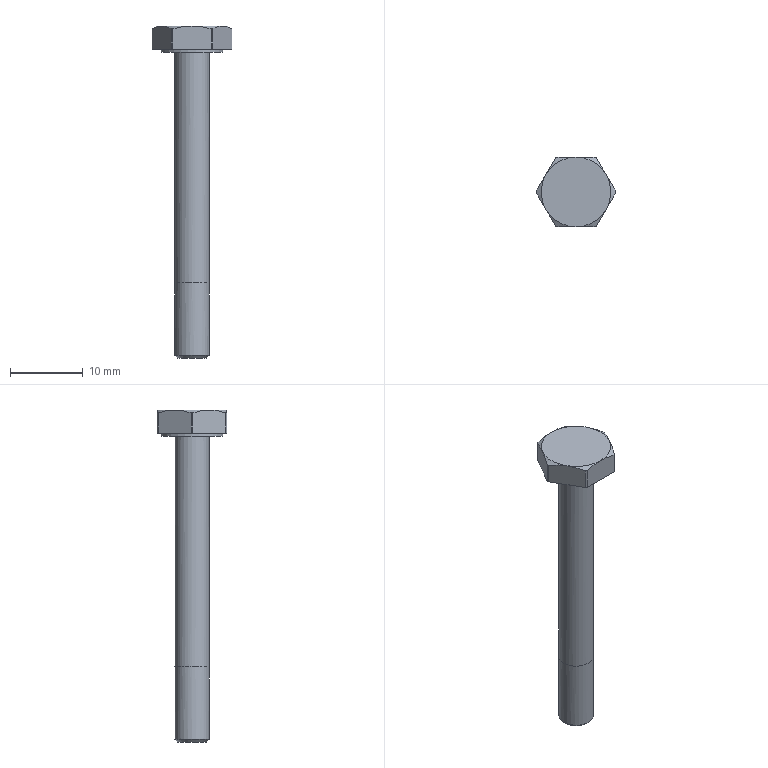Part | NX | features solid 2 | 1 solid | 26 faces | box 10.922 x 9.576 x 45.65 mm | volume 1023 mm3 | plane 10 | cylinder 9 | cone 7 | commonest cylinder face diameters 10.922 x6 4.763 x2 8.509 x1
STEP:
#1=CARTESIAN_POINT('',(-2.381,0.,-3.581));
#2=VERTEX_POINT('',#1);
#3=CARTESIAN_POINT('',(0.,0.,-3.581));
#4=DIRECTION('',(0.,0.,-1.));
#5=DIRECTION('',(-1.,0.,0.));
#6=AXIS2_PLACEMENT_3D('',#3,#4,#5);
#7=CIRCLE('',#6,2.381);
#8=EDGE_CURVE('',#2,#2,#7,.T.);
#9=ORIENTED_EDGE('',*,*,#8,.T.);
#10=EDGE_LOOP('',(#9));
#11=FACE_BOUND('',#10,.T.);
#12=CARTESIAN_POINT('',(-2.381,0.,-35.331));
#13=VERTEX_POINT('',#12);
#14=CARTESIAN_POINT('',(-1.866,1.866,-35.331));
#15=CARTESIAN_POINT('',(-2.639,0.,-35.331));
#16=CARTESIAN_POINT('',(-1.866,-1.866,-35.331));
#17=CARTESIAN_POINT('',(0.,-2.639,-35.331));
#18=CARTESIAN_POINT('',(1.866,-1.866,-35.331));
#19=CARTESIAN_POINT('',(2.639,0.,-35.331));
#20=CARTESIAN_POINT('',(1.866,1.866,-35.331));
#21=CARTESIAN_POINT('',(0.,2.639,-35.331));
#22=CARTESIAN_POINT('',(-1.866,1.866,-35.331));
#23=CARTESIAN_POINT('',(-2.639,0.,-35.331));
#24=CARTESIAN_POINT('',(-1.866,-1.866,-35.331));
#25=B_SPLINE_CURVE_WITH_KNOTS('',3,(#14,#15,#16,#17,#18,#19,#20,#21,#22,#23,#24),.UNSPECIFIED.,.T.,.F.,(1,1,1,1,1,1,1,1,1,1,1,1,1,1,1),(-0.375,-0.25,-0.125,0.,0.125,0.25,0.375,0.5,0.625,0.75,0.875,1.,1.125,1.25,1.375),.UNSPECIFIED.);
#26=EDGE_CURVE('',#13,#13,#25,.T.);
#27=ORIENTED_EDGE('',*,*,#26,.T.);
#28=EDGE_LOOP('',(#27));
#29=FACE_BOUND('',#28,.T.);
#30=CARTESIAN_POINT('',(0.,0.,0.));
#31=DIRECTION('',(0.,0.,-1.));
#32=DIRECTION('',(-1.,0.,0.));
#33=AXIS2_PLACEMENT_3D('',#30,#31,#32);
#34=CYLINDRICAL_SURFACE('',#33,2.381);
#35=ADVANCED_FACE('',(#11,#29),#34,.T.);
#36=CARTESIAN_POINT('',(2.627,4.788,-3.175));
#37=VERTEX_POINT('',#36);
#38=CARTESIAN_POINT('',(2.833,4.669,-3.175));
#39=VERTEX_POINT('',#38);
#40=CARTESIAN_POINT('',(0.,0.,-3.175));
#41=DIRECTION('',(0.,0.,-1.));
#42=DIRECTION('',(-1.,0.,0.));
#43=AXIS2_PLACEMENT_3D('',#40,#41,#42);
#44=CIRCLE('',#43,5.461);
#45=EDGE_CURVE('',#37,#39,#44,.T.);
#46=ORIENTED_EDGE('',*,*,#45,.F.);
#47=CARTESIAN_POINT('',(2.627,4.788,-0.3886));
#48=VERTEX_POINT('',#47);
#49=CARTESIAN_POINT('',(2.627,4.788,0.));
#50=DIRECTION('',(0.,0.,-1.));
#51=VECTOR('',#50,1000.);
#52=LINE('',#49,#51);
#53=EDGE_CURVE('',#37,#48,#52,.F.);
#54=ORIENTED_EDGE('',*,*,#53,.T.);
#55=CARTESIAN_POINT('',(2.833,4.669,-0.3886));
#56=VERTEX_POINT('',#55);
#57=CARTESIAN_POINT('',(0.,0.,-0.3886));
#58=DIRECTION('',(0.,0.,-1.));
#59=DIRECTION('',(-1.,0.,0.));
#60=AXIS2_PLACEMENT_3D('',#57,#58,#59);
#61=CIRCLE('',#60,5.461);
#62=EDGE_CURVE('',#48,#56,#61,.T.);
#63=ORIENTED_EDGE('',*,*,#62,.T.);
#64=CARTESIAN_POINT('',(2.833,4.669,0.));
#65=DIRECTION('',(0.,0.,-1.));
#66=VECTOR('',#65,1000.);
#67=LINE('',#64,#66);
#68=EDGE_CURVE('',#56,#39,#67,.T.);
#69=ORIENTED_EDGE('',*,*,#68,.T.);
#70=EDGE_LOOP('',(#46,#54,#63,#69));
#71=FACE_BOUND('',#70,.T.);
#72=CARTESIAN_POINT('',(0.,0.,0.));
#73=DIRECTION('',(0.,0.,-1.));
#74=DIRECTION('',(-1.,0.,0.));
#75=AXIS2_PLACEMENT_3D('',#72,#73,#74);
#76=CYLINDRICAL_SURFACE('',#75,5.461);
#77=ADVANCED_FACE('',(#71),#76,.T.);
#78=CARTESIAN_POINT('',(-2.833,4.669,-0.3886));
#79=VERTEX_POINT('',#78);
#80=CARTESIAN_POINT('',(-2.627,4.788,-0.3886));
#81=VERTEX_POINT('',#80);
#82=CARTESIAN_POINT('',(0.,0.,-0.3886));
#83=DIRECTION('',(0.,0.,-1.));
#84=DIRECTION('',(-1.,0.,0.));
#85=AXIS2_PLACEMENT_3D('',#82,#83,#84);
#86=CIRCLE('',#85,5.461);
#87=EDGE_CURVE('',#79,#81,#86,.T.);
#88=ORIENTED_EDGE('',*,*,#87,.T.);
#89=CARTESIAN_POINT('',(-2.627,4.788,-3.175));
#90=VERTEX_POINT('',#89);
#91=CARTESIAN_POINT('',(-2.627,4.788,0.));
#92=DIRECTION('',(0.,0.,-1.));
#93=VECTOR('',#92,1000.);
#94=LINE('',#91,#93);
#95=EDGE_CURVE('',#81,#90,#94,.T.);
#96=ORIENTED_EDGE('',*,*,#95,.T.);
#97=CARTESIAN_POINT('',(-2.833,4.669,-3.175));
#98=VERTEX_POINT('',#97);
#99=CARTESIAN_POINT('',(0.,0.,-3.175));
#100=DIRECTION('',(0.,0.,-1.));
#101=DIRECTION('',(-1.,0.,0.));
#102=AXIS2_PLACEMENT_3D('',#99,#100,#101);
#103=CIRCLE('',#102,5.461);
#104=EDGE_CURVE('',#98,#90,#103,.T.);
#105=ORIENTED_EDGE('',*,*,#104,.F.);
#106=CARTESIAN_POINT('',(-2.833,4.669,0.));
#107=DIRECTION('',(0.,0.,-1.));
#108=VECTOR('',#107,1000.);
#109=LINE('',#106,#108);
#110=EDGE_CURVE('',#98,#79,#109,.F.);
#111=ORIENTED_EDGE('',*,*,#110,.T.);
#112=EDGE_LOOP('',(#88,#96,#105,#111));
#113=FACE_BOUND('',#112,.T.);
#114=CARTESIAN_POINT('',(0.,0.,0.));
#115=DIRECTION('',(0.,0.,-1.));
#116=DIRECTION('',(-1.,0.,0.));
#117=AXIS2_PLACEMENT_3D('',#114,#115,#116);
#118=CYLINDRICAL_SURFACE('',#117,5.461);
#119=ADVANCED_FACE('',(#113),#118,.T.);
#120=CARTESIAN_POINT('',(-5.46,-0.1193,-0.3886));
#121=VERTEX_POINT('',#120);
#122=CARTESIAN_POINT('',(-5.46,0.1193,-0.3886));
#123=VERTEX_POINT('',#122);
#124=CARTESIAN_POINT('',(0.,0.,-0.3886));
#125=DIRECTION('',(0.,0.,-1.));
#126=DIRECTION('',(-1.,0.,0.));
#127=AXIS2_PLACEMENT_3D('',#124,#125,#126);
#128=CIRCLE('',#127,5.461);
#129=EDGE_CURVE('',#121,#123,#128,.T.);
#130=ORIENTED_EDGE('',*,*,#129,.T.);
#131=CARTESIAN_POINT('',(-5.46,0.1193,-3.175));
#132=VERTEX_POINT('',#131);
#133=CARTESIAN_POINT('',(-5.46,0.1193,0.));
#134=DIRECTION('',(0.,0.,-1.));
#135=VECTOR('',#134,1000.);
#136=LINE('',#133,#135);
#137=EDGE_CURVE('',#123,#132,#136,.T.);
#138=ORIENTED_EDGE('',*,*,#137,.T.);
#139=CARTESIAN_POINT('',(-5.46,-0.1193,-3.175));
#140=VERTEX_POINT('',#139);
#141=CARTESIAN_POINT('',(0.,0.,-3.175));
#142=DIRECTION('',(0.,0.,-1.));
#143=DIRECTION('',(-1.,0.,0.));
#144=AXIS2_PLACEMENT_3D('',#141,#142,#143);
#145=CIRCLE('',#144,5.461);
#146=EDGE_CURVE('',#140,#132,#145,.T.);
#147=ORIENTED_EDGE('',*,*,#146,.F.);
#148=CARTESIAN_POINT('',(-5.46,-0.1193,0.));
#149=DIRECTION('',(0.,0.,-1.));
#150=VECTOR('',#149,1000.);
#151=LINE('',#148,#150);
#152=EDGE_CURVE('',#140,#121,#151,.F.);
#153=ORIENTED_EDGE('',*,*,#152,.T.);
#154=EDGE_LOOP('',(#130,#138,#147,#153));
#155=FACE_BOUND('',#154,.T.);
#156=CARTESIAN_POINT('',(0.,0.,0.));
#157=DIRECTION('',(0.,0.,-1.));
#158=DIRECTION('',(-1.,0.,0.));
#159=AXIS2_PLACEMENT_3D('',#156,#157,#158);
#160=CYLINDRICAL_SURFACE('',#159,5.461);
#161=ADVANCED_FACE('',(#155),#160,.T.);
#162=CARTESIAN_POINT('',(-2.627,-4.788,-0.3886));
#163=VERTEX_POINT('',#162);
#164=CARTESIAN_POINT('',(-2.833,-4.669,-0.3886));
#165=VERTEX_POINT('',#164);
#166=CARTESIAN_POINT('',(0.,0.,-0.3886));
#167=DIRECTION('',(0.,0.,-1.));
#168=DIRECTION('',(-1.,0.,0.));
#169=AXIS2_PLACEMENT_3D('',#166,#167,#168);
#170=CIRCLE('',#169,5.461);
#171=EDGE_CURVE('',#163,#165,#170,.T.);
#172=ORIENTED_EDGE('',*,*,#171,.T.);
#173=CARTESIAN_POINT('',(-2.833,-4.669,-3.175));
#174=VERTEX_POINT('',#173);
#175=CARTESIAN_POINT('',(-2.833,-4.669,0.));
#176=DIRECTION('',(0.,0.,-1.));
#177=VECTOR('',#176,1000.);
#178=LINE('',#175,#177);
#179=EDGE_CURVE('',#165,#174,#178,.T.);
#180=ORIENTED_EDGE('',*,*,#179,.T.);
#181=CARTESIAN_POINT('',(-2.627,-4.788,-3.175));
#182=VERTEX_POINT('',#181);
#183=CARTESIAN_POINT('',(0.,0.,-3.175));
#184=DIRECTION('',(0.,0.,-1.));
#185=DIRECTION('',(-1.,0.,0.));
#186=AXIS2_PLACEMENT_3D('',#183,#184,#185);
#187=CIRCLE('',#186,5.461);
#188=EDGE_CURVE('',#182,#174,#187,.T.);
#189=ORIENTED_EDGE('',*,*,#188,.F.);
#190=CARTESIAN_POINT('',(-2.627,-4.788,0.));
#191=DIRECTION('',(0.,0.,-1.));
#192=VECTOR('',#191,1000.);
#193=LINE('',#190,#192);
#194=EDGE_CURVE('',#182,#163,#193,.F.);
#195=ORIENTED_EDGE('',*,*,#194,.T.);
#196=EDGE_LOOP('',(#172,#180,#189,#195));
#197=FACE_BOUND('',#196,.T.);
#198=CARTESIAN_POINT('',(0.,0.,0.));
#199=DIRECTION('',(0.,0.,-1.));
#200=DIRECTION('',(-1.,0.,0.));
#201=AXIS2_PLACEMENT_3D('',#198,#199,#200);
#202=CYLINDRICAL_SURFACE('',#201,5.461);
#203=ADVANCED_FACE('',(#197),#202,.T.);
#204=CARTESIAN_POINT('',(2.833,-4.669,-0.3886));
#205=VERTEX_POINT('',#204);
#206=CARTESIAN_POINT('',(2.627,-4.788,-0.3886));
#207=VERTEX_POINT('',#206);
#208=CARTESIAN_POINT('',(0.,0.,-0.3886));
#209=DIRECTION('',(0.,0.,-1.));
#210=DIRECTION('',(-1.,0.,0.));
#211=AXIS2_PLACEMENT_3D('',#208,#209,#210);
#212=CIRCLE('',#211,5.461);
#213=EDGE_CURVE('',#205,#207,#212,.T.);
#214=ORIENTED_EDGE('',*,*,#213,.T.);
#215=CARTESIAN_POINT('',(2.627,-4.788,-3.175));
#216=VERTEX_POINT('',#215);
#217=CARTESIAN_POINT('',(2.627,-4.788,0.));
#218=DIRECTION('',(0.,0.,-1.));
#219=VECTOR('',#218,1000.);
#220=LINE('',#217,#219);
#221=EDGE_CURVE('',#207,#216,#220,.T.);
#222=ORIENTED_EDGE('',*,*,#221,.T.);
#223=CARTESIAN_POINT('',(2.833,-4.669,-3.175));
#224=VERTEX_POINT('',#223);
#225=CARTESIAN_POINT('',(0.,0.,-3.175));
#226=DIRECTION('',(0.,0.,-1.));
#227=DIRECTION('',(-1.,0.,0.));
#228=AXIS2_PLACEMENT_3D('',#225,#226,#227);
#229=CIRCLE('',#228,5.461);
#230=EDGE_CURVE('',#224,#216,#229,.T.);
#231=ORIENTED_EDGE('',*,*,#230,.F.);
#232=CARTESIAN_POINT('',(2.833,-4.669,0.));
#233=DIRECTION('',(0.,0.,-1.));
#234=VECTOR('',#233,1000.);
#235=LINE('',#232,#234);
#236=EDGE_CURVE('',#224,#205,#235,.F.);
#237=ORIENTED_EDGE('',*,*,#236,.T.);
#238=EDGE_LOOP('',(#214,#222,#231,#237));
#239=FACE_BOUND('',#238,.T.);
#240=CARTESIAN_POINT('',(0.,0.,0.));
#241=DIRECTION('',(0.,0.,-1.));
#242=DIRECTION('',(-1.,0.,0.));
#243=AXIS2_PLACEMENT_3D('',#240,#241,#242);
#244=CYLINDRICAL_SURFACE('',#243,5.461);
#245=ADVANCED_FACE('',(#239),#244,.T.);
#246=ORIENTED_EDGE('',*,*,#62,.F.);
#247=CARTESIAN_POINT('',(0.,4.788,0.));
#248=VERTEX_POINT('',#247);
#249=CARTESIAN_POINT('',(0.,4.788,0.));
#250=CARTESIAN_POINT('',(0.8868,4.788,0.));
#251=CARTESIAN_POINT('',(1.776,4.788,-0.1525));
#252=CARTESIAN_POINT('',(2.627,4.788,-0.3886));
#253=B_SPLINE_CURVE_WITH_KNOTS('',3,(#249,#250,#251,#252),.UNSPECIFIED.,.F.,.F.,(4,4),(0.007722,0.01038),.UNSPECIFIED.);
#254=EDGE_CURVE('',#48,#248,#253,.F.);
#255=ORIENTED_EDGE('',*,*,#254,.T.);
#256=CARTESIAN_POINT('',(4.146,2.394,0.));
#257=VERTEX_POINT('',#256);
#258=CARTESIAN_POINT('',(0.,0.,0.));
#259=DIRECTION('',(0.,0.,-1.));
#260=DIRECTION('',(-1.,0.,0.));
#261=AXIS2_PLACEMENT_3D('',#258,#259,#260);
#262=CIRCLE('',#261,4.788);
#263=EDGE_CURVE('',#248,#257,#262,.T.);
#264=ORIENTED_EDGE('',*,*,#263,.T.);
#265=CARTESIAN_POINT('',(4.146,2.394,0.));
#266=CARTESIAN_POINT('',(3.703,3.163,0.));
#267=CARTESIAN_POINT('',(3.262,3.925,-0.1503));
#268=CARTESIAN_POINT('',(2.833,4.669,-0.3886));
#269=B_SPLINE_CURVE_WITH_KNOTS('',3,(#265,#266,#267,#268),.UNSPECIFIED.,.F.,.F.,(4,4),(0.002655,0.005296),.UNSPECIFIED.);
#270=EDGE_CURVE('',#257,#56,#269,.T.);
#271=ORIENTED_EDGE('',*,*,#270,.T.);
#272=EDGE_LOOP('',(#246,#255,#264,#271));
#273=FACE_BOUND('',#272,.T.);
#274=CARTESIAN_POINT('',(0.,0.,-0.3886));
#275=DIRECTION('',(0.,0.,-1.));
#276=DIRECTION('',(-1.,0.,0.));
#277=AXIS2_PLACEMENT_3D('',#274,#275,#276);
#278=CONICAL_SURFACE('',#277,5.461,1.047);
#279=ADVANCED_FACE('',(#273),#278,.T.);
#280=CARTESIAN_POINT('',(-4.146,2.394,0.));
#281=VERTEX_POINT('',#280);
#282=CARTESIAN_POINT('',(0.,0.,0.));
#283=DIRECTION('',(0.,0.,-1.));
#284=DIRECTION('',(-1.,0.,0.));
#285=AXIS2_PLACEMENT_3D('',#282,#283,#284);
#286=CIRCLE('',#285,4.788);
#287=EDGE_CURVE('',#281,#248,#286,.T.);
#288=ORIENTED_EDGE('',*,*,#287,.T.);
#289=CARTESIAN_POINT('',(-2.627,4.788,-0.3886));
#290=CARTESIAN_POINT('',(-1.77,4.788,-0.1508));
#291=CARTESIAN_POINT('',(-0.8866,4.788,0.));
#292=CARTESIAN_POINT('',(0.,4.788,0.));
#293=B_SPLINE_CURVE_WITH_KNOTS('',3,(#289,#290,#291,#292),.UNSPECIFIED.,.F.,.F.,(4,4),(0.005068,0.007722),.UNSPECIFIED.);
#294=EDGE_CURVE('',#248,#81,#293,.F.);
#295=ORIENTED_EDGE('',*,*,#294,.T.);
#296=ORIENTED_EDGE('',*,*,#87,.F.);
#297=CARTESIAN_POINT('',(-2.833,4.669,-0.3886));
#298=CARTESIAN_POINT('',(-3.264,3.923,-0.1495));
#299=CARTESIAN_POINT('',(-3.7,3.167,0.));
#300=CARTESIAN_POINT('',(-4.146,2.394,0.));
#301=B_SPLINE_CURVE_WITH_KNOTS('',3,(#297,#298,#299,#300),.UNSPECIFIED.,.F.,.F.,(4,4),(0.00000074,0.002655),.UNSPECIFIED.);
#302=EDGE_CURVE('',#79,#281,#301,.T.);
#303=ORIENTED_EDGE('',*,*,#302,.T.);
#304=EDGE_LOOP('',(#288,#295,#296,#303));
#305=FACE_BOUND('',#304,.T.);
#306=CARTESIAN_POINT('',(0.,0.,-0.3886));
#307=DIRECTION('',(0.,0.,-1.));
#308=DIRECTION('',(-1.,0.,0.));
#309=AXIS2_PLACEMENT_3D('',#306,#307,#308);
#310=CONICAL_SURFACE('',#309,5.461,1.047);
#311=ADVANCED_FACE('',(#305),#310,.T.);
#312=CARTESIAN_POINT('',(-4.146,-2.394,0.));
#313=VERTEX_POINT('',#312);
#314=CARTESIAN_POINT('',(0.,0.,0.));
#315=DIRECTION('',(0.,0.,-1.));
#316=DIRECTION('',(-1.,0.,0.));
#317=AXIS2_PLACEMENT_3D('',#314,#315,#316);
#318=CIRCLE('',#317,4.788);
#319=EDGE_CURVE('',#313,#281,#318,.T.);
#320=ORIENTED_EDGE('',*,*,#319,.T.);
#321=CARTESIAN_POINT('',(-4.146,2.394,0.));
#322=CARTESIAN_POINT('',(-4.59,1.625,0.));
#323=CARTESIAN_POINT('',(-5.031,0.8625,-0.1503));
#324=CARTESIAN_POINT('',(-5.46,0.1193,-0.3886));
#325=B_SPLINE_CURVE_WITH_KNOTS('',3,(#321,#322,#323,#324),.UNSPECIFIED.,.F.,.F.,(4,4),(0.002655,0.005296),.UNSPECIFIED.);
#326=EDGE_CURVE('',#281,#123,#325,.T.);
#327=ORIENTED_EDGE('',*,*,#326,.T.);
#328=ORIENTED_EDGE('',*,*,#129,.F.);
#329=CARTESIAN_POINT('',(-5.46,-0.1193,-0.3886));
#330=CARTESIAN_POINT('',(-5.029,-0.8651,-0.1495));
#331=CARTESIAN_POINT('',(-4.593,-1.621,0.));
#332=CARTESIAN_POINT('',(-4.146,-2.394,0.));
#333=B_SPLINE_CURVE_WITH_KNOTS('',3,(#329,#330,#331,#332),.UNSPECIFIED.,.F.,.F.,(4,4),(0.00000074,0.002655),.UNSPECIFIED.);
#334=EDGE_CURVE('',#121,#313,#333,.T.);
#335=ORIENTED_EDGE('',*,*,#334,.T.);
#336=EDGE_LOOP('',(#320,#327,#328,#335));
#337=FACE_BOUND('',#336,.T.);
#338=CARTESIAN_POINT('',(0.,0.,-0.3886));
#339=DIRECTION('',(0.,0.,-1.));
#340=DIRECTION('',(-1.,0.,0.));
#341=AXIS2_PLACEMENT_3D('',#338,#339,#340);
#342=CONICAL_SURFACE('',#341,5.461,1.047);
#343=ADVANCED_FACE('',(#337),#342,.T.);
#344=CARTESIAN_POINT('',(0.,-4.788,0.));
#345=VERTEX_POINT('',#344);
#346=CARTESIAN_POINT('',(0.,0.,0.));
#347=DIRECTION('',(0.,0.,-1.));
#348=DIRECTION('',(-1.,0.,0.));
#349=AXIS2_PLACEMENT_3D('',#346,#347,#348);
#350=CIRCLE('',#349,4.788);
#351=EDGE_CURVE('',#345,#313,#350,.T.);
#352=ORIENTED_EDGE('',*,*,#351,.T.);
#353=CARTESIAN_POINT('',(-4.146,-2.394,0.));
#354=CARTESIAN_POINT('',(-3.703,-3.163,0.));
#355=CARTESIAN_POINT('',(-3.262,-3.925,-0.1503));
#356=CARTESIAN_POINT('',(-2.833,-4.669,-0.3886));
#357=B_SPLINE_CURVE_WITH_KNOTS('',3,(#353,#354,#355,#356),.UNSPECIFIED.,.F.,.F.,(4,4),(0.002655,0.005296),.UNSPECIFIED.);
#358=EDGE_CURVE('',#313,#165,#357,.T.);
#359=ORIENTED_EDGE('',*,*,#358,.T.);
#360=ORIENTED_EDGE('',*,*,#171,.F.);
#361=CARTESIAN_POINT('',(-2.627,-4.788,-0.3886));
#362=CARTESIAN_POINT('',(-1.77,-4.788,-0.1508));
#363=CARTESIAN_POINT('',(-0.8866,-4.788,0.));
#364=CARTESIAN_POINT('',(0.,-4.788,0.));
#365=B_SPLINE_CURVE_WITH_KNOTS('',3,(#361,#362,#363,#364),.UNSPECIFIED.,.F.,.F.,(4,4),(0.005068,0.007722),.UNSPECIFIED.);
#366=EDGE_CURVE('',#163,#345,#365,.T.);
#367=ORIENTED_EDGE('',*,*,#366,.T.);
#368=EDGE_LOOP('',(#352,#359,#360,#367));
#369=FACE_BOUND('',#368,.T.);
#370=CARTESIAN_POINT('',(0.,0.,-0.3886));
#371=DIRECTION('',(0.,0.,-1.));
#372=DIRECTION('',(-1.,0.,0.));
#373=AXIS2_PLACEMENT_3D('',#370,#371,#372);
#374=CONICAL_SURFACE('',#373,5.461,1.047);
#375=ADVANCED_FACE('',(#369),#374,.T.);
#376=CARTESIAN_POINT('',(4.146,-2.394,0.));
#377=VERTEX_POINT('',#376);
#378=CARTESIAN_POINT('',(0.,0.,0.));
#379=DIRECTION('',(0.,0.,-1.));
#380=DIRECTION('',(-1.,0.,0.));
#381=AXIS2_PLACEMENT_3D('',#378,#379,#380);
#382=CIRCLE('',#381,4.788);
#383=EDGE_CURVE('',#377,#345,#382,.T.);
#384=ORIENTED_EDGE('',*,*,#383,.T.);
#385=CARTESIAN_POINT('',(0.,-4.788,0.));
#386=CARTESIAN_POINT('',(0.8868,-4.788,0.));
#387=CARTESIAN_POINT('',(1.776,-4.788,-0.1525));
#388=CARTESIAN_POINT('',(2.627,-4.788,-0.3886));
#389=B_SPLINE_CURVE_WITH_KNOTS('',3,(#385,#386,#387,#388),.UNSPECIFIED.,.F.,.F.,(4,4),(0.007722,0.01038),.UNSPECIFIED.);
#390=EDGE_CURVE('',#345,#207,#389,.T.);
#391=ORIENTED_EDGE('',*,*,#390,.T.);
#392=ORIENTED_EDGE('',*,*,#213,.F.);
#393=CARTESIAN_POINT('',(2.833,-4.669,-0.3886));
#394=CARTESIAN_POINT('',(3.264,-3.923,-0.1495));
#395=CARTESIAN_POINT('',(3.7,-3.167,0.));
#396=CARTESIAN_POINT('',(4.146,-2.394,0.));
#397=B_SPLINE_CURVE_WITH_KNOTS('',3,(#393,#394,#395,#396),.UNSPECIFIED.,.F.,.F.,(4,4),(0.00000074,0.002655),.UNSPECIFIED.);
#398=EDGE_CURVE('',#205,#377,#397,.T.);
#399=ORIENTED_EDGE('',*,*,#398,.T.);
#400=EDGE_LOOP('',(#384,#391,#392,#399));
#401=FACE_BOUND('',#400,.T.);
#402=CARTESIAN_POINT('',(0.,0.,-0.3886));
#403=DIRECTION('',(0.,0.,-1.));
#404=DIRECTION('',(-1.,0.,0.));
#405=AXIS2_PLACEMENT_3D('',#402,#403,#404);
#406=CONICAL_SURFACE('',#405,5.461,1.047);
#407=ADVANCED_FACE('',(#401),#406,.T.);
#408=ORIENTED_EDGE('',*,*,#104,.T.);
#409=CARTESIAN_POINT('',(4.255,4.788,-3.175));
#410=DIRECTION('',(1.,0.,0.));
#411=VECTOR('',#410,1000.);
#412=LINE('',#409,#411);
#413=EDGE_CURVE('',#90,#37,#412,.T.);
#414=ORIENTED_EDGE('',*,*,#413,.T.);
#415=ORIENTED_EDGE('',*,*,#45,.T.);
#416=CARTESIAN_POINT('',(5.46,0.1193,-3.175));
#417=VERTEX_POINT('',#416);
#418=CARTESIAN_POINT('',(5.21,0.5517,-3.175));
#419=DIRECTION('',(0.5,-0.866,0.));
#420=VECTOR('',#419,1000.);
#421=LINE('',#418,#420);
#422=EDGE_CURVE('',#39,#417,#421,.T.);
#423=ORIENTED_EDGE('',*,*,#422,.T.);
#424=CARTESIAN_POINT('',(5.46,-0.1193,-3.175));
#425=VERTEX_POINT('',#424);
#426=CARTESIAN_POINT('',(0.,0.,-3.175));
#427=DIRECTION('',(0.,0.,-1.));
#428=DIRECTION('',(-1.,0.,0.));
#429=AXIS2_PLACEMENT_3D('',#426,#427,#428);
#430=CIRCLE('',#429,5.461);
#431=EDGE_CURVE('',#417,#425,#430,.T.);
#432=ORIENTED_EDGE('',*,*,#431,.T.);
#433=CARTESIAN_POINT('',(5.21,-0.5517,-3.175));
#434=DIRECTION('',(-0.5,-0.866,0.));
#435=VECTOR('',#434,1000.);
#436=LINE('',#433,#435);
#437=EDGE_CURVE('',#425,#224,#436,.T.);
#438=ORIENTED_EDGE('',*,*,#437,.T.);
#439=ORIENTED_EDGE('',*,*,#230,.T.);
#440=CARTESIAN_POINT('',(4.255,-4.788,-3.175));
#441=DIRECTION('',(-1.,0.,0.));
#442=VECTOR('',#441,1000.);
#443=LINE('',#440,#442);
#444=EDGE_CURVE('',#216,#182,#443,.T.);
#445=ORIENTED_EDGE('',*,*,#444,.T.);
#446=ORIENTED_EDGE('',*,*,#188,.T.);
#447=CARTESIAN_POINT('',(-3.083,-4.236,-3.175));
#448=DIRECTION('',(-0.5,0.866,0.));
#449=VECTOR('',#448,1000.);
#450=LINE('',#447,#449);
#451=EDGE_CURVE('',#174,#140,#450,.T.);
#452=ORIENTED_EDGE('',*,*,#451,.T.);
#453=ORIENTED_EDGE('',*,*,#146,.T.);
#454=CARTESIAN_POINT('',(-3.083,4.236,-3.175));
#455=DIRECTION('',(0.5,0.866,0.));
#456=VECTOR('',#455,1000.);
#457=LINE('',#454,#456);
#458=EDGE_CURVE('',#132,#98,#457,.T.);
#459=ORIENTED_EDGE('',*,*,#458,.T.);
#460=EDGE_LOOP('',(#408,#414,#415,#423,#432,#438,#439,#445,#446,#452,#453,#459));
#461=FACE_BOUND('',#460,.T.);
#462=CARTESIAN_POINT('',(-4.255,0.,-3.175));
#463=VERTEX_POINT('',#462);
#464=CARTESIAN_POINT('',(0.,0.,-3.175));
#465=DIRECTION('',(0.,0.,-1.));
#466=DIRECTION('',(-1.,0.,0.));
#467=AXIS2_PLACEMENT_3D('',#464,#465,#466);
#468=CIRCLE('',#467,4.255);
#469=EDGE_CURVE('',#463,#463,#468,.T.);
#470=ORIENTED_EDGE('',*,*,#469,.F.);
#471=EDGE_LOOP('',(#470));
#472=FACE_BOUND('',#471,.T.);
#473=CARTESIAN_POINT('',(4.255,0.,-3.175));
#474=DIRECTION('',(0.,0.,-1.));
#475=DIRECTION('',(-1.,0.,0.));
#476=AXIS2_PLACEMENT_3D('',#473,#474,#475);
#477=PLANE('',#476);
#478=ADVANCED_FACE('',(#461,#472),#477,.T.);
#479=CARTESIAN_POINT('',(5.46,0.1193,-0.3886));
#480=VERTEX_POINT('',#479);
#481=CARTESIAN_POINT('',(5.46,-0.1193,-0.3886));
#482=VERTEX_POINT('',#481);
#483=CARTESIAN_POINT('',(0.,0.,-0.3886));
#484=DIRECTION('',(0.,0.,-1.));
#485=DIRECTION('',(-1.,0.,0.));
#486=AXIS2_PLACEMENT_3D('',#483,#484,#485);
#487=CIRCLE('',#486,5.461);
#488=EDGE_CURVE('',#480,#482,#487,.T.);
#489=ORIENTED_EDGE('',*,*,#488,.T.);
#490=CARTESIAN_POINT('',(5.46,-0.1193,0.));
#491=DIRECTION('',(0.,0.,-1.));
#492=VECTOR('',#491,1000.);
#493=LINE('',#490,#492);
#494=EDGE_CURVE('',#482,#425,#493,.T.);
#495=ORIENTED_EDGE('',*,*,#494,.T.);
#496=ORIENTED_EDGE('',*,*,#431,.F.);
#497=CARTESIAN_POINT('',(5.46,0.1193,0.));
#498=DIRECTION('',(0.,0.,-1.));
#499=VECTOR('',#498,1000.);
#500=LINE('',#497,#499);
#501=EDGE_CURVE('',#417,#480,#500,.F.);
#502=ORIENTED_EDGE('',*,*,#501,.T.);
#503=EDGE_LOOP('',(#489,#495,#496,#502));
#504=FACE_BOUND('',#503,.T.);
#505=CARTESIAN_POINT('',(0.,0.,0.));
#506=DIRECTION('',(0.,0.,-1.));
#507=DIRECTION('',(-1.,0.,0.));
#508=AXIS2_PLACEMENT_3D('',#505,#506,#507);
#509=CYLINDRICAL_SURFACE('',#508,5.461);
#510=ADVANCED_FACE('',(#504),#509,.T.);
#511=CARTESIAN_POINT('',(0.,0.,0.));
#512=DIRECTION('',(0.,0.,-1.));
#513=DIRECTION('',(-1.,0.,0.));
#514=AXIS2_PLACEMENT_3D('',#511,#512,#513);
#515=CIRCLE('',#514,4.788);
#516=EDGE_CURVE('',#257,#377,#515,.T.);
#517=ORIENTED_EDGE('',*,*,#516,.T.);
#518=CARTESIAN_POINT('',(4.146,-2.394,0.));
#519=CARTESIAN_POINT('',(4.59,-1.625,0.));
#520=CARTESIAN_POINT('',(5.031,-0.8625,-0.1503));
#521=CARTESIAN_POINT('',(5.46,-0.1193,-0.3886));
#522=B_SPLINE_CURVE_WITH_KNOTS('',3,(#518,#519,#520,#521),.UNSPECIFIED.,.F.,.F.,(4,4),(0.002655,0.005296),.UNSPECIFIED.);
#523=EDGE_CURVE('',#377,#482,#522,.T.);
#524=ORIENTED_EDGE('',*,*,#523,.T.);
#525=ORIENTED_EDGE('',*,*,#488,.F.);
#526=CARTESIAN_POINT('',(5.46,0.1193,-0.3886));
#527=CARTESIAN_POINT('',(5.029,0.8651,-0.1495));
#528=CARTESIAN_POINT('',(4.593,1.621,0.));
#529=CARTESIAN_POINT('',(4.146,2.394,0.));
#530=B_SPLINE_CURVE_WITH_KNOTS('',3,(#526,#527,#528,#529),.UNSPECIFIED.,.F.,.F.,(4,4),(0.00000074,0.002655),.UNSPECIFIED.);
#531=EDGE_CURVE('',#480,#257,#530,.T.);
#532=ORIENTED_EDGE('',*,*,#531,.T.);
#533=EDGE_LOOP('',(#517,#524,#525,#532));
#534=FACE_BOUND('',#533,.T.);
#535=CARTESIAN_POINT('',(0.,0.,-0.3886));
#536=DIRECTION('',(0.,0.,-1.));
#537=DIRECTION('',(-1.,0.,0.));
#538=AXIS2_PLACEMENT_3D('',#535,#536,#537);
#539=CONICAL_SURFACE('',#538,5.461,1.047);
#540=ADVANCED_FACE('',(#534),#539,.T.);
#541=ORIENTED_EDGE('',*,*,#287,.F.);
#542=ORIENTED_EDGE('',*,*,#319,.F.);
#543=ORIENTED_EDGE('',*,*,#351,.F.);
#544=ORIENTED_EDGE('',*,*,#383,.F.);
#545=ORIENTED_EDGE('',*,*,#516,.F.);
#546=ORIENTED_EDGE('',*,*,#263,.F.);
#547=EDGE_LOOP('',(#541,#542,#543,#544,#545,#546));
#548=FACE_BOUND('',#547,.T.);
#549=CARTESIAN_POINT('',(4.788,0.,0.));
#550=DIRECTION('',(0.,0.,1.));
#551=DIRECTION('',(1.,0.,0.));
#552=AXIS2_PLACEMENT_3D('',#549,#550,#551);
#553=PLANE('',#552);
#554=ADVANCED_FACE('',(#548),#553,.T.);
#555=CARTESIAN_POINT('',(-2.,0.,-45.65));
#556=VERTEX_POINT('',#555);
#557=CARTESIAN_POINT('',(0.,0.,-45.65));
#558=DIRECTION('',(0.,0.,-1.));
#559=DIRECTION('',(-1.,0.,0.));
#560=AXIS2_PLACEMENT_3D('',#557,#558,#559);
#561=CIRCLE('',#560,2.);
#562=EDGE_CURVE('',#556,#556,#561,.T.);
#563=ORIENTED_EDGE('',*,*,#562,.T.);
#564=EDGE_LOOP('',(#563));
#565=FACE_BOUND('',#564,.T.);
#566=CARTESIAN_POINT('',(0.,0.,-45.65));
#567=DIRECTION('',(0.,0.,-1.));
#568=DIRECTION('',(-1.,0.,0.));
#569=AXIS2_PLACEMENT_3D('',#566,#567,#568);
#570=PLANE('',#569);
#571=ADVANCED_FACE('',(#565),#570,.T.);
#572=CARTESIAN_POINT('',(-2.381,0.,-45.269));
#573=VERTEX_POINT('',#572);
#574=CARTESIAN_POINT('',(0.,0.,-45.269));
#575=DIRECTION('',(0.,0.,-1.));
#576=DIRECTION('',(-1.,0.,0.));
#577=AXIS2_PLACEMENT_3D('',#574,#575,#576);
#578=CIRCLE('',#577,2.381);
#579=EDGE_CURVE('',#573,#573,#578,.T.);
#580=ORIENTED_EDGE('',*,*,#579,.T.);
#581=EDGE_LOOP('',(#580));
#582=FACE_BOUND('',#581,.T.);
#583=ORIENTED_EDGE('',*,*,#562,.F.);
#584=EDGE_LOOP('',(#583));
#585=FACE_BOUND('',#584,.T.);
#586=CARTESIAN_POINT('',(0.,0.,-45.65));
#587=DIRECTION('',(0.,0.,1.));
#588=DIRECTION('',(1.,0.,0.));
#589=AXIS2_PLACEMENT_3D('',#586,#587,#588);
#590=CONICAL_SURFACE('',#589,2.,0.7854);
#591=ADVANCED_FACE('',(#582,#585),#590,.T.);
#592=ORIENTED_EDGE('',*,*,#26,.F.);
#593=EDGE_LOOP('',(#592));
#594=FACE_BOUND('',#593,.T.);
#595=ORIENTED_EDGE('',*,*,#579,.F.);
#596=EDGE_LOOP('',(#595));
#597=FACE_BOUND('',#596,.T.);
#598=CARTESIAN_POINT('',(0.,0.,0.));
#599=DIRECTION('',(0.,0.,-1.));
#600=DIRECTION('',(-1.,0.,0.));
#601=AXIS2_PLACEMENT_3D('',#598,#599,#600);
#602=CYLINDRICAL_SURFACE('',#601,2.381);
#603=ADVANCED_FACE('',(#594,#597),#602,.T.);
#604=CARTESIAN_POINT('',(-4.255,0.,-3.581));
#605=VERTEX_POINT('',#604);
#606=CARTESIAN_POINT('',(0.,0.,-3.581));
#607=DIRECTION('',(0.,0.,-1.));
#608=DIRECTION('',(-1.,0.,0.));
#609=AXIS2_PLACEMENT_3D('',#606,#607,#608);
#610=CIRCLE('',#609,4.255);
#611=EDGE_CURVE('',#605,#605,#610,.T.);
#612=ORIENTED_EDGE('',*,*,#611,.T.);
#613=EDGE_LOOP('',(#612));
#614=FACE_BOUND('',#613,.T.);
#615=ORIENTED_EDGE('',*,*,#8,.F.);
#616=EDGE_LOOP('',(#615));
#617=FACE_BOUND('',#616,.T.);
#618=CARTESIAN_POINT('',(2.381,0.,-3.581));
#619=DIRECTION('',(0.,0.,-1.));
#620=DIRECTION('',(-1.,0.,0.));
#621=AXIS2_PLACEMENT_3D('',#618,#619,#620);
#622=PLANE('',#621);
#623=ADVANCED_FACE('',(#614,#617),#622,.T.);
#624=ORIENTED_EDGE('',*,*,#469,.T.);
#625=EDGE_LOOP('',(#624));
#626=FACE_BOUND('',#625,.T.);
#627=ORIENTED_EDGE('',*,*,#611,.F.);
#628=EDGE_LOOP('',(#627));
#629=FACE_BOUND('',#628,.T.);
#630=CARTESIAN_POINT('',(0.,0.,0.));
#631=DIRECTION('',(0.,0.,-1.));
#632=DIRECTION('',(-1.,0.,0.));
#633=AXIS2_PLACEMENT_3D('',#630,#631,#632);
#634=CYLINDRICAL_SURFACE('',#633,4.255);
#635=ADVANCED_FACE('',(#626,#629),#634,.T.);
#636=ORIENTED_EDGE('',*,*,#422,.F.);
#637=ORIENTED_EDGE('',*,*,#68,.F.);
#638=ORIENTED_EDGE('',*,*,#270,.F.);
#639=ORIENTED_EDGE('',*,*,#531,.F.);
#640=ORIENTED_EDGE('',*,*,#501,.F.);
#641=EDGE_LOOP('',(#636,#637,#638,#639,#640));
#642=FACE_BOUND('',#641,.T.);
#643=CARTESIAN_POINT('',(5.529,0.,-50.215));
#644=DIRECTION('',(0.866,0.5,0.));
#645=DIRECTION('',(-0.5,0.866,0.));
#646=AXIS2_PLACEMENT_3D('',#643,#644,#645);
#647=PLANE('',#646);
#648=ADVANCED_FACE('',(#642),#647,.T.);
#649=ORIENTED_EDGE('',*,*,#437,.F.);
#650=ORIENTED_EDGE('',*,*,#494,.F.);
#651=ORIENTED_EDGE('',*,*,#523,.F.);
#652=ORIENTED_EDGE('',*,*,#398,.F.);
#653=ORIENTED_EDGE('',*,*,#236,.F.);
#654=EDGE_LOOP('',(#649,#650,#651,#652,#653));
#655=FACE_BOUND('',#654,.T.);
#656=CARTESIAN_POINT('',(2.764,-4.788,-50.215));
#657=DIRECTION('',(0.866,-0.5,0.));
#658=DIRECTION('',(0.5,0.866,0.));
#659=AXIS2_PLACEMENT_3D('',#656,#657,#658);
#660=PLANE('',#659);
#661=ADVANCED_FACE('',(#655),#660,.T.);
#662=ORIENTED_EDGE('',*,*,#444,.F.);
#663=ORIENTED_EDGE('',*,*,#221,.F.);
#664=ORIENTED_EDGE('',*,*,#390,.F.);
#665=ORIENTED_EDGE('',*,*,#366,.F.);
#666=ORIENTED_EDGE('',*,*,#194,.F.);
#667=EDGE_LOOP('',(#662,#663,#664,#665,#666));
#668=FACE_BOUND('',#667,.T.);
#669=CARTESIAN_POINT('',(-2.764,-4.788,-50.215));
#670=DIRECTION('',(0.,-1.,0.));
#671=DIRECTION('',(0.,0.,-1.));
#672=AXIS2_PLACEMENT_3D('',#669,#670,#671);
#673=PLANE('',#672);
#674=ADVANCED_FACE('',(#668),#673,.T.);
#675=ORIENTED_EDGE('',*,*,#451,.F.);
#676=ORIENTED_EDGE('',*,*,#179,.F.);
#677=ORIENTED_EDGE('',*,*,#358,.F.);
#678=ORIENTED_EDGE('',*,*,#334,.F.);
#679=ORIENTED_EDGE('',*,*,#152,.F.);
#680=EDGE_LOOP('',(#675,#676,#677,#678,#679));
#681=FACE_BOUND('',#680,.T.);
#682=CARTESIAN_POINT('',(-5.529,0.,-50.215));
#683=DIRECTION('',(-0.866,-0.5,0.));
#684=DIRECTION('',(0.5,-0.866,0.));
#685=AXIS2_PLACEMENT_3D('',#682,#683,#684);
#686=PLANE('',#685);
#687=ADVANCED_FACE('',(#681),#686,.T.);
#688=ORIENTED_EDGE('',*,*,#458,.F.);
#689=ORIENTED_EDGE('',*,*,#137,.F.);
#690=ORIENTED_EDGE('',*,*,#326,.F.);
#691=ORIENTED_EDGE('',*,*,#302,.F.);
#692=ORIENTED_EDGE('',*,*,#110,.F.);
#693=EDGE_LOOP('',(#688,#689,#690,#691,#692));
#694=FACE_BOUND('',#693,.T.);
#695=CARTESIAN_POINT('',(-2.764,4.788,-50.215));
#696=DIRECTION('',(-0.866,0.5,0.));
#697=DIRECTION('',(-0.5,-0.866,0.));
#698=AXIS2_PLACEMENT_3D('',#695,#696,#697);
#699=PLANE('',#698);
#700=ADVANCED_FACE('',(#694),#699,.T.);
#701=ORIENTED_EDGE('',*,*,#413,.F.);
#702=ORIENTED_EDGE('',*,*,#95,.F.);
#703=ORIENTED_EDGE('',*,*,#294,.F.);
#704=ORIENTED_EDGE('',*,*,#254,.F.);
#705=ORIENTED_EDGE('',*,*,#53,.F.);
#706=EDGE_LOOP('',(#701,#702,#703,#704,#705));
#707=FACE_BOUND('',#706,.T.);
#708=CARTESIAN_POINT('',(2.764,4.788,-50.215));
#709=DIRECTION('',(0.,1.,0.));
#710=DIRECTION('',(0.,0.,1.));
#711=AXIS2_PLACEMENT_3D('',#708,#709,#710);
#712=PLANE('',#711);
#713=ADVANCED_FACE('',(#707),#712,.T.);
#714=CLOSED_SHELL('',(#35,#77,#119,#161,#203,#245,#279,#311,#343,#375,#407,#478,#510,#540,#554,#571,#591,#603,#623,#635,#648,#661,#674,#687,#700,#713));
#715=MANIFOLD_SOLID_BREP('',#714);
#716=(LENGTH_UNIT()NAMED_UNIT(*)SI_UNIT(.MILLI.,.METRE.));
#717=UNCERTAINTY_MEASURE_WITH_UNIT(LENGTH_MEASURE(0.0508),#716,'','');
#718=(NAMED_UNIT(*)PLANE_ANGLE_UNIT()SI_UNIT($,.RADIAN.));
#719=(NAMED_UNIT(*)SI_UNIT($,.STERADIAN.)SOLID_ANGLE_UNIT());
#720=(GEOMETRIC_REPRESENTATION_CONTEXT(3)GLOBAL_UNCERTAINTY_ASSIGNED_CONTEXT((#717))GLOBAL_UNIT_ASSIGNED_CONTEXT((#716,#718,#719))REPRESENTATION_CONTEXT('',''));
#721=ADVANCED_BREP_SHAPE_REPRESENTATION('',(#715),#720);